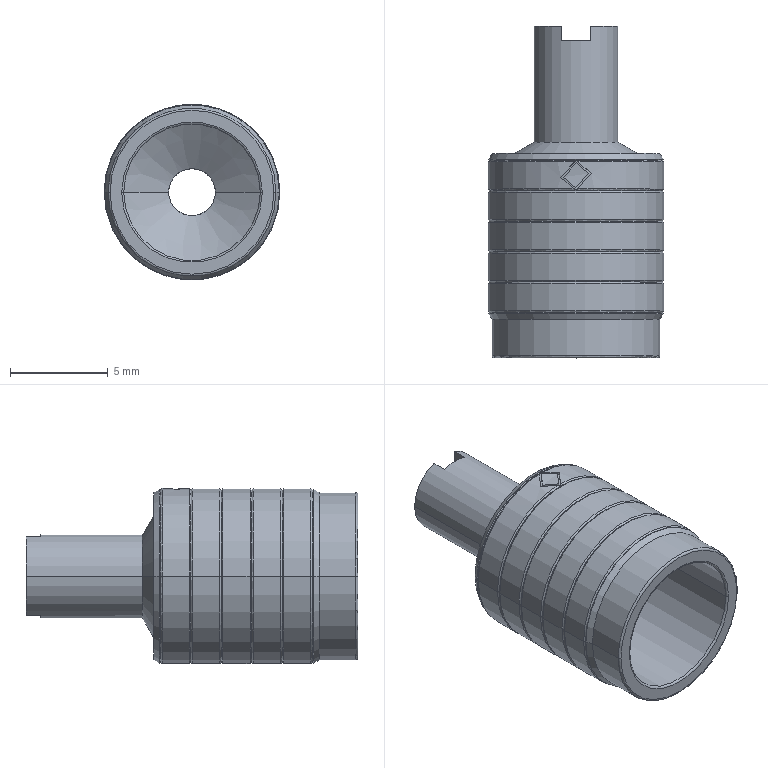Part | STEP file | VALVE_6PARTV11 | 1 solid | 77 faces | box 9 x 17 x 9 mm | volume 343.749 mm3 | spline 22 | cylinder 21 | plane 18 | torus 8 | cone 8 | commonest cylinder face diameters 9 x12 2.4 x2 4.3 x2 7 x2 8.6 x2 8.84 x1